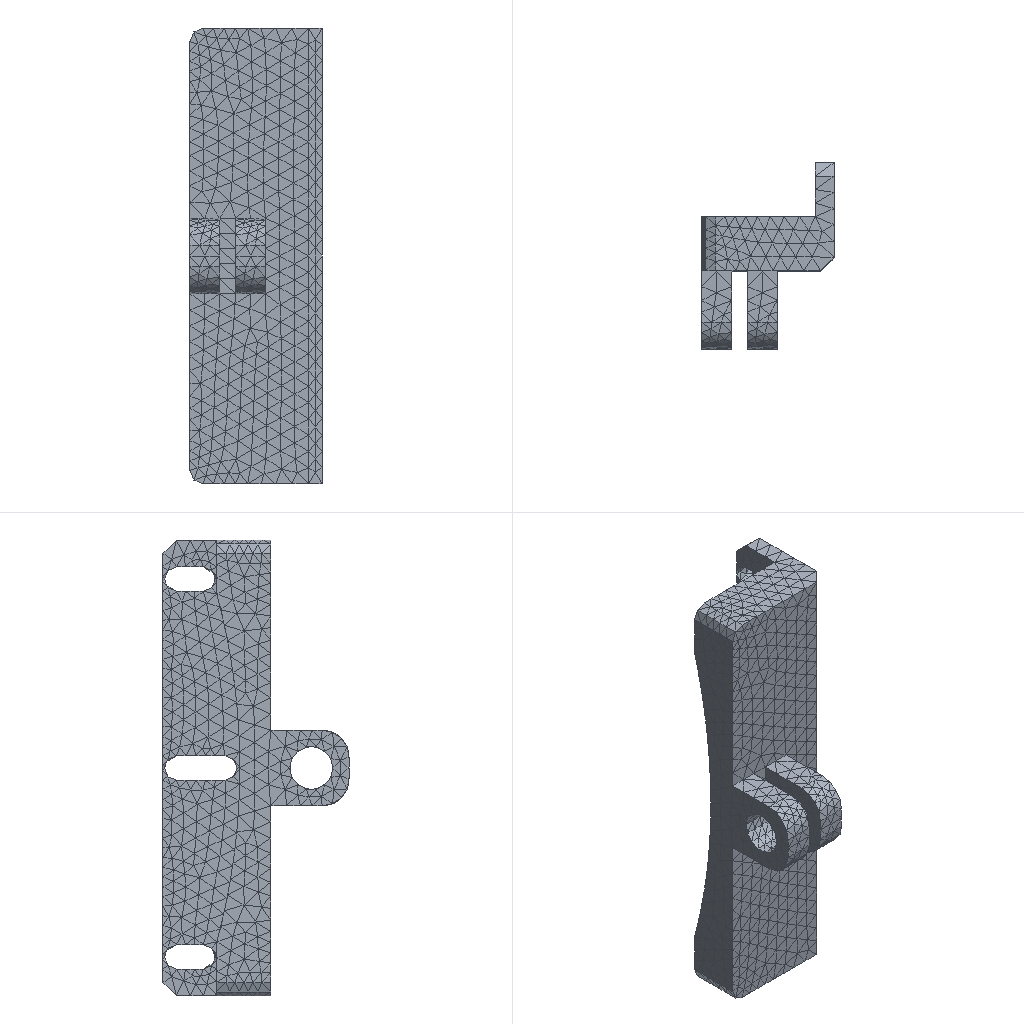Simulation study | nx simcenter
Set-up summary:
category,name,step,type,value,unit,region
solver,nx_nastran (Simcenter)
units,not stated in the deck,,not stated
analysis,deck,,static,static
analysis,solution,,SOL,101
load_step,SUBCASE 1,1,SUBCASE,SPC=1 LOAD=2
load_step,requested,,,1
mesh,nodes,,,11420
mesh,elements,,,5947
element_type,CTETRA,,solid,5947
load,nodal force total,,FX,-2499999.906,model units
load,nodal force total,,FY,0.0,model units
load,nodal force total,,FZ,0.0,model units
load,load commands in deck,,count,757
bc,support commands in deck,,count,392
analysis,NX solution 0,,Structural,Linear Statics - Single Constraint
check,setup vs results,,match,every grid point's frame and coordinates and every element id; grid points of CTETRA elements
Nastran input file, long lists of numbers shortened:
$*$$$$$$$$$$$$$$$$$$$$$$$$$$$$$$$$$$$$$$$$$$$$$$$$$$$$$$$$$$$$$$$$$
$*
$*                    NX v10.0.0.24 TRANSLATOR
$*                    FOR NX NASTRAN VERSION 10.0
$ (33 more lines like these left out)
ASSIGN OUTPUT2='148_sim1-solution_1.op2' UNIT=12
$*
$*$$$$$$$$$$$$$$$$$$$$$$$$$$$$$$$$$$$
$*
$* EXECUTIVE CONTROL
$*
$*$$$$$$$$$$$$$$$$$$$$$$$$$$$$$$$$$$$
$*
ID,NASTRAN,148_sim1-solution_1
SOL 101
CEND
$*
$*$$$$$$$$$$$$$$$$$$$$$$$$$$$$$$$$$$$
$*
$* CASE CONTROL
$*
$*$$$$$$$$$$$$$$$$$$$$$$$$$$$$$$$$$$$
$*
TITLE = Solution 1
ECHO = NONE
SPC = 1
OUTPUT
BCRESULTS(TRACTION,FORCE,PLOT) = ALL
DISPLACEMENT(PLOT) = ALL
ESE(PLOT) = ALL
FORCE(PLOT,CORNER) = ALL
OLOAD(PLOT) = ALL
SPCFORCES(PLOT) = ALL
STRAIN(PLOT,FIBER,CORNER) = ALL
STRESS(PLOT,CORNER) = ALL
$*  NX Step: Subcase - Static Loads 1
SUBCASE 1
LABEL = Subcase - Static Loads 1
LOAD = 2
$*
$*$$$$$$$$$$$$$$$$$$$$$$$$$$$$$$$$$$$
$*
$* BULK DATA
$*
$*$$$$$$$$$$$$$$$$$$$$$$$$$$$$$$$$$$$
$*
BEGIN BULK
$*
$* PARAM CARDS
$*
PARAM      K6ROT100.0000
PARAM     OIBULK     YES
PARAM    OMACHPR     YES
PARAM       POST      -2
PARAM    POSTEXT     YES
PARAM    UNITSYS   MN-MM
$*
$* GRID CARDS
$*
GRID*              11327               0-5.000000000E+00-1.400000000E+01+
*       4.0000000000E+00               0
GRID*              11328               0-5.000000000E+00-1.400000000E+01+
*       -4.000000000E+00               0
$ (22836 more lines like these left out)
$*
$* ELEMENT CARDS
$*
$*  NX Mesh Collector: Solid(1)
$*  NX Mesh: 3d_mesh(1)
CTETRA         1       1       1       2       3       4     276     277+
+            278     279     280     281
CTETRA         2       1       2    7412       5       3     282     283+
+            284     277     285     286
$ (11890 more lines like these left out)
$*
$* PROPERTY CARDS
$*
$*  NX Property: PSOLID1
PSOLID         1       1       0                           SMECH
$*
$* MATERIAL CARDS
$*
$*  NX Material: 3A21
MAT1           17.3119+7        0.3300002.7300-62.1355-5
MATT1          1       1               2               3
TABLEM1        1                                                        +
+        20.00007.3119+7 21.11007.3119+7 23.89007.3119+7 37.78007.3119+7+
+        51.67007.3119+7 65.56007.2429+7 79.44007.2429+7 93.33007.1739+7+
+       107.22007.1049+7121.11007.0359+7135.00006.9670+7148.89006.8980+7+
+       162.78006.8290+7176.67006.6910+7190.56006.6221+7204.44006.4841+7+
+       218.33006.3461+7232.22006.1392+7246.11006.0012+7260.00005.8633+7+
+       273.89005.7253+7287.78005.5184+7301.67005.3804+7315.56005.1735+7+
+       329.44004.9665+7343.33004.7596+7357.22004.6216+7371.11004.4147+7+
+           ENDT
TABLEM1        2                                                        +
+        20.00000.330000 21.11000.330000    ENDT
TABLEM1        3                                                        +
+        20.00002.1600-5 93.33002.2500-5107.22002.2662-5121.11002.2824-5+
+       135.00002.2968-5148.89002.3130-5162.78002.3274-5176.67002.3418-5+
+       190.56002.3544-5204.44002.3688-5218.33002.3814-5232.22002.3958-5+
+       246.11002.4066-5260.00002.4192-5273.89002.4300-5287.78002.4408-5+
+       301.67002.4498-5315.56002.4606-5329.44002.4696-5343.33002.4786-5+
+       357.22002.4876-5371.11002.4984-5385.00002.5110-5398.89002.5254-5+
+       412.78002.5398-5426.67002.5560-5    ENDT
$*
$* LOAD AND CONSTRAINT CARDS
$*
$*  NX Load and Constraint: Fixed(1)
SPC            1    9738  123456  0.0000
SPC            1    9739  123456  0.0000
SPC            1    9740  123456  0.0000
SPC            1    9741  123456  0.0000
$ (388 more lines like these left out)
$*  NX Load and Constraint: Force(1)
FORCE          2    8976       0 1021.83-1.00000  0.0000  0.0000
FORCE          2    8977       0 3647.90-1.00000  0.0000  0.0000
FORCE          2    8978       0 3571.30-1.00000  0.0000  0.0000
FORCE          2    8979       0 4380.55-1.00000  0.0000  0.0000
$ (753 more lines like these left out)
ENDDATA d335f14a
Results summary:
result,analysis,,,static
result,last_loadstep,,,1
result,primary field,,,displacements
result,reaction total,,FX,2499999.75,model units
result,reaction total,,FY,-0.4785,model units
result,reaction total,,FZ,-0.0152,model units
result,NX solution 0,,loadcases,1,mm